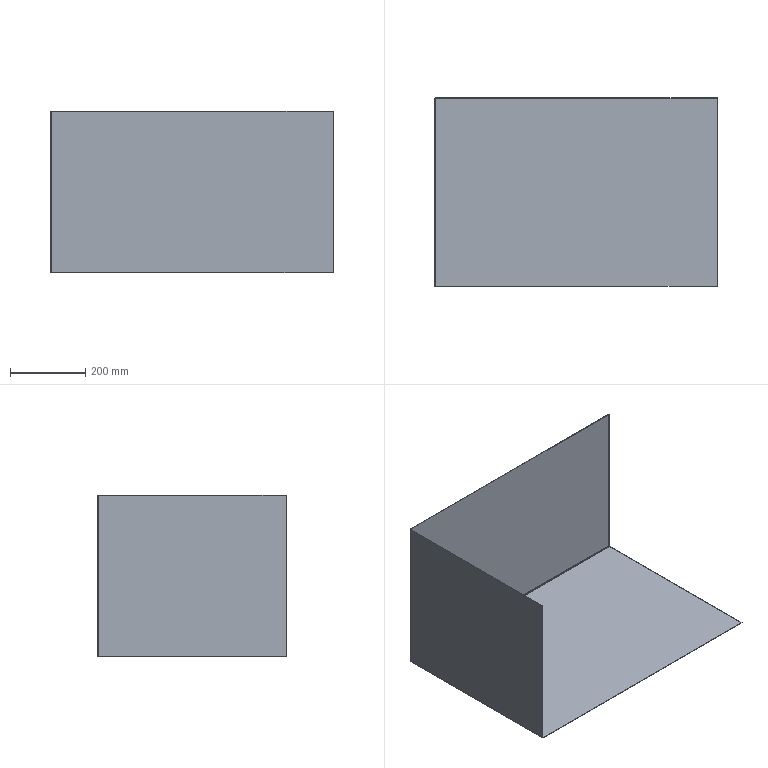Part | 1 solid | 22 faces | box 750 x 500 x 430 mm | volume 1090375 mm3 | plane 16 | cylinder 4 | spline 2 | commonest cylinder face diameters 1.473 x2 3.873 x2
STEP:
#1=CARTESIAN_POINT('',(-373.063,-250.,-1.2));
#2=VERTEX_POINT('',#1);
#3=CARTESIAN_POINT('',(-373.063,248.063,-1.2));
#4=VERTEX_POINT('',#3);
#5=CARTESIAN_POINT('',(-373.063,-250.,-1.2));
#6=DIRECTION('',(0.,1.,0.));
#7=VECTOR('',#6,1000.);
#8=LINE('',#5,#7);
#9=EDGE_CURVE('',#2,#4,#8,.T.);
#10=ORIENTED_EDGE('',*,*,#9,.T.);
#11=CARTESIAN_POINT('',(375.,248.063,-1.2));
#12=VERTEX_POINT('',#11);
#13=CARTESIAN_POINT('',(-373.093,248.063,-1.2));
#14=DIRECTION('',(1.,0.,0.));
#15=VECTOR('',#14,1000.);
#16=LINE('',#13,#15);
#17=EDGE_CURVE('',#4,#12,#16,.T.);
#18=ORIENTED_EDGE('',*,*,#17,.T.);
#19=CARTESIAN_POINT('',(375.,-250.,-1.2));
#20=VERTEX_POINT('',#19);
#21=CARTESIAN_POINT('',(375.,250.,-1.2));
#22=DIRECTION('',(0.,1.,0.));
#23=VECTOR('',#22,1000.);
#24=LINE('',#21,#23);
#25=EDGE_CURVE('',#20,#12,#24,.T.);
#26=ORIENTED_EDGE('',*,*,#25,.F.);
#27=CARTESIAN_POINT('',(-375.,-250.,-1.2));
#28=DIRECTION('',(1.,0.,0.));
#29=VECTOR('',#28,1000.);
#30=LINE('',#27,#29);
#31=EDGE_CURVE('',#2,#20,#30,.T.);
#32=ORIENTED_EDGE('',*,*,#31,.F.);
#33=EDGE_LOOP('',(#10,#18,#26,#32));
#34=FACE_OUTER_BOUND('',#33,.T.);
#35=CARTESIAN_POINT('',(0.,0.,-1.2));
#36=DIRECTION('',(0.,0.,1.));
#37=DIRECTION('',(1.,0.,0.));
#38=AXIS2_PLACEMENT_3D('',#35,#36,#37);
#39=PLANE('',#38);
#40=ADVANCED_FACE('',(#34),#39,.F.);
#41=CARTESIAN_POINT('',(-373.063,248.063,0.));
#42=VERTEX_POINT('',#41);
#43=CARTESIAN_POINT('',(375.,248.063,0.));
#44=VERTEX_POINT('',#43);
#45=CARTESIAN_POINT('',(-373.093,248.063,0.));
#46=DIRECTION('',(1.,0.,0.));
#47=VECTOR('',#46,1000.);
#48=LINE('',#45,#47);
#49=EDGE_CURVE('',#42,#44,#48,.T.);
#50=ORIENTED_EDGE('',*,*,#49,.F.);
#51=CARTESIAN_POINT('',(-373.063,-250.,0.));
#52=VERTEX_POINT('',#51);
#53=CARTESIAN_POINT('',(-373.063,-250.,0.));
#54=DIRECTION('',(0.,1.,0.));
#55=VECTOR('',#54,1000.);
#56=LINE('',#53,#55);
#57=EDGE_CURVE('',#52,#42,#56,.T.);
#58=ORIENTED_EDGE('',*,*,#57,.F.);
#59=CARTESIAN_POINT('',(375.,-250.,0.));
#60=VERTEX_POINT('',#59);
#61=CARTESIAN_POINT('',(-375.,-250.,0.));
#62=DIRECTION('',(1.,0.,0.));
#63=VECTOR('',#62,1000.);
#64=LINE('',#61,#63);
#65=EDGE_CURVE('',#52,#60,#64,.T.);
#66=ORIENTED_EDGE('',*,*,#65,.T.);
#67=CARTESIAN_POINT('',(375.,250.,0.));
#68=DIRECTION('',(0.,1.,0.));
#69=VECTOR('',#68,1000.);
#70=LINE('',#67,#69);
#71=EDGE_CURVE('',#60,#44,#70,.T.);
#72=ORIENTED_EDGE('',*,*,#71,.T.);
#73=EDGE_LOOP('',(#50,#58,#66,#72));
#74=FACE_OUTER_BOUND('',#73,.T.);
#75=CARTESIAN_POINT('',(0.,0.,0.));
#76=DIRECTION('',(0.,0.,1.));
#77=DIRECTION('',(1.,0.,0.));
#78=AXIS2_PLACEMENT_3D('',#75,#76,#77);
#79=PLANE('',#78);
#80=ADVANCED_FACE('',(#74),#79,.T.);
#81=ORIENTED_EDGE('',*,*,#65,.F.);
#82=CARTESIAN_POINT('',(-373.063,-250.,0.));
#83=DIRECTION('',(0.,0.,-1.));
#84=VECTOR('',#83,1000.);
#85=LINE('',#82,#84);
#86=EDGE_CURVE('',#52,#2,#85,.T.);
#87=ORIENTED_EDGE('',*,*,#86,.T.);
#88=ORIENTED_EDGE('',*,*,#31,.T.);
#89=CARTESIAN_POINT('',(375.,-250.,-1.2));
#90=DIRECTION('',(0.,0.,1.));
#91=VECTOR('',#90,1000.);
#92=LINE('',#89,#91);
#93=EDGE_CURVE('',#20,#60,#92,.T.);
#94=ORIENTED_EDGE('',*,*,#93,.T.);
#95=EDGE_LOOP('',(#81,#87,#88,#94));
#96=FACE_OUTER_BOUND('',#95,.T.);
#97=CARTESIAN_POINT('',(-375.,-250.,-1.2));
#98=DIRECTION('',(0.,-1.,0.));
#99=DIRECTION('',(0.,0.,-1.));
#100=AXIS2_PLACEMENT_3D('',#97,#98,#99);
#101=PLANE('',#100);
#102=ADVANCED_FACE('',(#96),#101,.T.);
#103=CARTESIAN_POINT('',(375.,248.063,0.));
#104=DIRECTION('',(0.,0.,-1.));
#105=VECTOR('',#104,1000.);
#106=LINE('',#103,#105);
#107=EDGE_CURVE('',#44,#12,#106,.T.);
#108=ORIENTED_EDGE('',*,*,#107,.F.);
#109=ORIENTED_EDGE('',*,*,#71,.F.);
#110=ORIENTED_EDGE('',*,*,#93,.F.);
#111=ORIENTED_EDGE('',*,*,#25,.T.);
#112=EDGE_LOOP('',(#108,#109,#110,#111));
#113=FACE_OUTER_BOUND('',#112,.T.);
#114=CARTESIAN_POINT('',(375.,250.,-1.2));
#115=DIRECTION('',(1.,0.,0.));
#116=DIRECTION('',(0.,1.,0.));
#117=AXIS2_PLACEMENT_3D('',#114,#115,#116);
#118=PLANE('',#117);
#119=ADVANCED_FACE('',(#113),#118,.T.);
#120=CARTESIAN_POINT('',(375.,248.8,0.7366));
#121=VERTEX_POINT('',#120);
#122=CARTESIAN_POINT('',(375.,250.,0.7366));
#123=VERTEX_POINT('',#122);
#124=CARTESIAN_POINT('',(375.,250.,0.7366));
#125=DIRECTION('',(0.,1.,0.));
#126=VECTOR('',#125,1000.);
#127=LINE('',#124,#126);
#128=EDGE_CURVE('',#121,#123,#127,.T.);
#129=ORIENTED_EDGE('',*,*,#128,.F.);
#130=CARTESIAN_POINT('',(375.,248.063,0.7366));
#131=DIRECTION('',(1.,0.,0.));
#132=DIRECTION('',(0.,0.,1.));
#133=AXIS2_PLACEMENT_3D('',#130,#131,#132);
#134=CIRCLE('',#133,0.7366);
#135=EDGE_CURVE('',#44,#121,#134,.T.);
#136=ORIENTED_EDGE('',*,*,#135,.F.);
#137=ORIENTED_EDGE('',*,*,#107,.T.);
#138=CARTESIAN_POINT('',(375.,248.063,0.7366));
#139=DIRECTION('',(1.,0.,0.));
#140=DIRECTION('',(0.,0.,1.));
#141=AXIS2_PLACEMENT_3D('',#138,#139,#140);
#142=CIRCLE('',#141,1.937);
#143=EDGE_CURVE('',#12,#123,#142,.T.);
#144=ORIENTED_EDGE('',*,*,#143,.T.);
#145=EDGE_LOOP('',(#129,#136,#137,#144));
#146=FACE_OUTER_BOUND('',#145,.T.);
#147=CARTESIAN_POINT('',(375.,248.063,0.7366));
#148=DIRECTION('',(1.,0.,0.));
#149=DIRECTION('',(0.,0.,-1.));
#150=AXIS2_PLACEMENT_3D('',#147,#148,#149);
#151=PLANE('',#150);
#152=ADVANCED_FACE('',(#146),#151,.T.);
#153=CARTESIAN_POINT('',(-373.093,248.8,0.7366));
#154=VERTEX_POINT('',#153);
#155=CARTESIAN_POINT('',(-373.093,248.8,0.7366));
#156=CARTESIAN_POINT('',(-373.088,248.8,0.5438));
#157=CARTESIAN_POINT('',(-373.083,248.721,0.3521));
#158=CARTESIAN_POINT('',(-373.073,248.448,0.07939));
#159=CARTESIAN_POINT('',(-373.068,248.256,0.));
#160=CARTESIAN_POINT('',(-373.063,248.063,0.));
#161=B_SPLINE_CURVE_WITH_KNOTS('',3,(#155,#156,#157,#158,#159,#160),.UNSPECIFIED.,.F.,.F.,(4,2,4),(0.,0.5,1.),.UNSPECIFIED.);
#162=EDGE_CURVE('',#154,#42,#161,.T.);
#163=ORIENTED_EDGE('',*,*,#162,.F.);
#164=CARTESIAN_POINT('',(-373.093,250.,0.7366));
#165=VERTEX_POINT('',#164);
#166=CARTESIAN_POINT('',(-373.093,248.8,0.7366));
#167=DIRECTION('',(0.,-1.,0.));
#168=VECTOR('',#167,1000.);
#169=LINE('',#166,#168);
#170=EDGE_CURVE('',#165,#154,#169,.T.);
#171=ORIENTED_EDGE('',*,*,#170,.F.);
#172=CARTESIAN_POINT('',(-373.093,250.,0.7366));
#173=CARTESIAN_POINT('',(-373.09,250.,0.4831));
#174=CARTESIAN_POINT('',(-373.088,249.95,0.2297));
#175=CARTESIAN_POINT('',(-373.083,249.756,-0.2387));
#176=CARTESIAN_POINT('',(-373.081,249.612,-0.4535));
#177=CARTESIAN_POINT('',(-373.076,249.254,-0.812));
#178=CARTESIAN_POINT('',(-373.073,249.039,-0.9556));
#179=CARTESIAN_POINT('',(-373.068,248.57,-1.15));
#180=CARTESIAN_POINT('',(-373.066,248.317,-1.2));
#181=CARTESIAN_POINT('',(-373.063,248.063,-1.2));
#182=B_SPLINE_CURVE_WITH_KNOTS('',3,(#172,#173,#174,#175,#176,#177,#178,#179,#180,#181),.UNSPECIFIED.,.F.,.F.,(4,2,2,2,4),(0.,0.25,0.5,0.75,1.),.UNSPECIFIED.);
#183=EDGE_CURVE('',#165,#4,#182,.T.);
#184=ORIENTED_EDGE('',*,*,#183,.T.);
#185=CARTESIAN_POINT('',(-373.063,248.063,0.));
#186=DIRECTION('',(0.,0.,-1.));
#187=VECTOR('',#186,1000.);
#188=LINE('',#185,#187);
#189=EDGE_CURVE('',#42,#4,#188,.T.);
#190=ORIENTED_EDGE('',*,*,#189,.F.);
#191=EDGE_LOOP('',(#163,#171,#184,#190));
#192=FACE_OUTER_BOUND('',#191,.T.);
#193=CARTESIAN_POINT('',(-373.093,250.012,0.7366));
#194=CARTESIAN_POINT('',(-373.09,250.012,0.4815));
#195=CARTESIAN_POINT('',(-373.088,249.961,0.2266));
#196=CARTESIAN_POINT('',(-373.083,249.766,-0.2448));
#197=CARTESIAN_POINT('',(-373.081,249.622,-0.4609));
#198=CARTESIAN_POINT('',(-373.076,249.261,-0.8216));
#199=CARTESIAN_POINT('',(-373.073,249.045,-0.9661));
#200=CARTESIAN_POINT('',(-373.068,248.573,-1.161));
#201=CARTESIAN_POINT('',(-373.066,248.319,-1.212));
#202=CARTESIAN_POINT('',(-373.063,248.063,-1.212));
#203=CARTESIAN_POINT('',(-373.093,250.,0.7366));
#204=CARTESIAN_POINT('',(-373.09,250.,0.4831));
#205=CARTESIAN_POINT('',(-373.088,249.95,0.2297));
#206=CARTESIAN_POINT('',(-373.083,249.756,-0.2387));
#207=CARTESIAN_POINT('',(-373.081,249.612,-0.4535));
#208=CARTESIAN_POINT('',(-373.076,249.254,-0.812));
#209=CARTESIAN_POINT('',(-373.073,249.039,-0.9556));
#210=CARTESIAN_POINT('',(-373.068,248.57,-1.15));
#211=CARTESIAN_POINT('',(-373.066,248.317,-1.2));
#212=CARTESIAN_POINT('',(-373.063,248.063,-1.2));
#213=CARTESIAN_POINT('',(-373.093,248.8,0.7366));
#214=CARTESIAN_POINT('',(-373.09,248.8,0.6402));
#215=CARTESIAN_POINT('',(-373.088,248.781,0.5438));
#216=CARTESIAN_POINT('',(-373.083,248.707,0.3656));
#217=CARTESIAN_POINT('',(-373.081,248.652,0.2839));
#218=CARTESIAN_POINT('',(-373.076,248.516,0.1476));
#219=CARTESIAN_POINT('',(-373.073,248.434,0.09297));
#220=CARTESIAN_POINT('',(-373.068,248.256,0.01917));
#221=CARTESIAN_POINT('',(-373.066,248.16,0.));
#222=CARTESIAN_POINT('',(-373.063,248.063,0.));
#223=CARTESIAN_POINT('',(-373.093,248.788,0.7366));
#224=CARTESIAN_POINT('',(-373.09,248.788,0.6417));
#225=CARTESIAN_POINT('',(-373.088,248.769,0.547));
#226=CARTESIAN_POINT('',(-373.083,248.696,0.3717));
#227=CARTESIAN_POINT('',(-373.081,248.643,0.2914));
#228=CARTESIAN_POINT('',(-373.076,248.509,0.1573));
#229=CARTESIAN_POINT('',(-373.073,248.428,0.1036));
#230=CARTESIAN_POINT('',(-373.068,248.253,0.03098));
#231=CARTESIAN_POINT('',(-373.066,248.158,0.01212));
#232=CARTESIAN_POINT('',(-373.063,248.063,0.01212));
#233=B_SPLINE_SURFACE_WITH_KNOTS('',1,3,((#193,#194,#195,#196,#197,#198,#199,#200,#201,#202),(#203,#204,#205,#206,#207,#208,#209,#210,#211,#212),(#213,#214,#215,#216,#217,#218,#219,#220,#221,#222),(#223,#224,#225,#226,#227,#228,#229,#230,#231,#232)),.UNSPECIFIED.,.F.,.F.,.F.,(2,1,1,2),(4,2,2,2,4),(-0.01,0.,1.,1.01),(0.,0.25,0.5,0.75,1.),.UNSPECIFIED.);
#234=ADVANCED_FACE('',(#192),#233,.F.);
#235=ORIENTED_EDGE('',*,*,#17,.F.);
#236=ORIENTED_EDGE('',*,*,#183,.F.);
#237=CARTESIAN_POINT('',(0.,250.,0.7366));
#238=DIRECTION('',(-1.,0.,0.));
#239=VECTOR('',#238,1000.);
#240=LINE('',#237,#239);
#241=EDGE_CURVE('',#123,#165,#240,.T.);
#242=ORIENTED_EDGE('',*,*,#241,.F.);
#243=ORIENTED_EDGE('',*,*,#143,.F.);
#244=EDGE_LOOP('',(#235,#236,#242,#243));
#245=FACE_OUTER_BOUND('',#244,.T.);
#246=CARTESIAN_POINT('',(-373.093,248.063,0.7366));
#247=DIRECTION('',(-1.,0.,0.));
#248=DIRECTION('',(0.,1.,0.));
#249=AXIS2_PLACEMENT_3D('',#246,#247,#248);
#250=CYLINDRICAL_SURFACE('',#249,1.937);
#251=ADVANCED_FACE('',(#245),#250,.T.);
#252=ORIENTED_EDGE('',*,*,#49,.T.);
#253=ORIENTED_EDGE('',*,*,#135,.T.);
#254=CARTESIAN_POINT('',(375.,248.8,0.7366));
#255=DIRECTION('',(-1.,0.,0.));
#256=VECTOR('',#255,1000.);
#257=LINE('',#254,#256);
#258=EDGE_CURVE('',#121,#154,#257,.T.);
#259=ORIENTED_EDGE('',*,*,#258,.T.);
#260=ORIENTED_EDGE('',*,*,#162,.T.);
#261=EDGE_LOOP('',(#252,#253,#259,#260));
#262=FACE_OUTER_BOUND('',#261,.T.);
#263=CARTESIAN_POINT('',(-373.093,248.063,0.7366));
#264=DIRECTION('',(-1.,0.,0.));
#265=DIRECTION('',(0.,1.,0.));
#266=AXIS2_PLACEMENT_3D('',#263,#264,#265);
#267=CYLINDRICAL_SURFACE('',#266,0.7366);
#268=ADVANCED_FACE('',(#262),#267,.F.);
#269=CARTESIAN_POINT('',(375.,248.8,428.8));
#270=VERTEX_POINT('',#269);
#271=CARTESIAN_POINT('',(375.,248.8,0.));
#272=DIRECTION('',(0.,0.,1.));
#273=VECTOR('',#272,1000.);
#274=LINE('',#271,#273);
#275=EDGE_CURVE('',#121,#270,#274,.T.);
#276=ORIENTED_EDGE('',*,*,#275,.F.);
#277=ORIENTED_EDGE('',*,*,#128,.T.);
#278=CARTESIAN_POINT('',(375.,250.,428.8));
#279=VERTEX_POINT('',#278);
#280=CARTESIAN_POINT('',(375.,250.,428.8));
#281=DIRECTION('',(0.,0.,1.));
#282=VECTOR('',#281,1000.);
#283=LINE('',#280,#282);
#284=EDGE_CURVE('',#123,#279,#283,.T.);
#285=ORIENTED_EDGE('',*,*,#284,.T.);
#286=CARTESIAN_POINT('',(375.,250.,428.8));
#287=DIRECTION('',(0.,-1.,0.));
#288=VECTOR('',#287,1000.);
#289=LINE('',#286,#288);
#290=EDGE_CURVE('',#279,#270,#289,.T.);
#291=ORIENTED_EDGE('',*,*,#290,.T.);
#292=EDGE_LOOP('',(#276,#277,#285,#291));
#293=FACE_OUTER_BOUND('',#292,.T.);
#294=CARTESIAN_POINT('',(375.,250.,428.8));
#295=DIRECTION('',(1.,0.,0.));
#296=DIRECTION('',(0.,0.,-1.));
#297=AXIS2_PLACEMENT_3D('',#294,#295,#296);
#298=PLANE('',#297);
#299=ADVANCED_FACE('',(#293),#298,.T.);
#300=CARTESIAN_POINT('',(-373.093,250.,428.8));
#301=VERTEX_POINT('',#300);
#302=CARTESIAN_POINT('',(-373.093,250.,0.));
#303=DIRECTION('',(0.,0.,-1.));
#304=VECTOR('',#303,1000.);
#305=LINE('',#302,#304);
#306=EDGE_CURVE('',#301,#165,#305,.T.);
#307=ORIENTED_EDGE('',*,*,#306,.F.);
#308=CARTESIAN_POINT('',(-375.,250.,428.8));
#309=DIRECTION('',(-1.,0.,0.));
#310=VECTOR('',#309,1000.);
#311=LINE('',#308,#310);
#312=EDGE_CURVE('',#279,#301,#311,.T.);
#313=ORIENTED_EDGE('',*,*,#312,.F.);
#314=ORIENTED_EDGE('',*,*,#284,.F.);
#315=ORIENTED_EDGE('',*,*,#241,.T.);
#316=EDGE_LOOP('',(#307,#313,#314,#315));
#317=FACE_OUTER_BOUND('',#316,.T.);
#318=CARTESIAN_POINT('',(0.,250.,0.));
#319=DIRECTION('',(0.,1.,0.));
#320=DIRECTION('',(0.,0.,1.));
#321=AXIS2_PLACEMENT_3D('',#318,#319,#320);
#322=PLANE('',#321);
#323=ADVANCED_FACE('',(#317),#322,.T.);
#324=CARTESIAN_POINT('',(-373.093,248.8,428.8));
#325=VERTEX_POINT('',#324);
#326=CARTESIAN_POINT('',(0.,248.8,428.8));
#327=DIRECTION('',(-1.,0.,0.));
#328=VECTOR('',#327,1000.);
#329=LINE('',#326,#328);
#330=EDGE_CURVE('',#270,#325,#329,.T.);
#331=ORIENTED_EDGE('',*,*,#330,.T.);
#332=CARTESIAN_POINT('',(-373.093,248.8,0.));
#333=DIRECTION('',(0.,0.,1.));
#334=VECTOR('',#333,1000.);
#335=LINE('',#332,#334);
#336=EDGE_CURVE('',#154,#325,#335,.T.);
#337=ORIENTED_EDGE('',*,*,#336,.F.);
#338=ORIENTED_EDGE('',*,*,#258,.F.);
#339=ORIENTED_EDGE('',*,*,#275,.T.);
#340=EDGE_LOOP('',(#331,#337,#338,#339));
#341=FACE_OUTER_BOUND('',#340,.T.);
#342=CARTESIAN_POINT('',(0.,248.8,0.));
#343=DIRECTION('',(0.,1.,0.));
#344=DIRECTION('',(0.,0.,1.));
#345=AXIS2_PLACEMENT_3D('',#342,#343,#344);
#346=PLANE('',#345);
#347=ADVANCED_FACE('',(#341),#346,.F.);
#348=CARTESIAN_POINT('',(-373.093,248.8,428.8));
#349=DIRECTION('',(0.,1.,0.));
#350=VECTOR('',#349,1000.);
#351=LINE('',#348,#350);
#352=EDGE_CURVE('',#325,#301,#351,.T.);
#353=ORIENTED_EDGE('',*,*,#352,.F.);
#354=ORIENTED_EDGE('',*,*,#330,.F.);
#355=ORIENTED_EDGE('',*,*,#290,.F.);
#356=ORIENTED_EDGE('',*,*,#312,.T.);
#357=EDGE_LOOP('',(#353,#354,#355,#356));
#358=FACE_OUTER_BOUND('',#357,.T.);
#359=CARTESIAN_POINT('',(-375.,250.,428.8));
#360=DIRECTION('',(0.,0.,1.));
#361=DIRECTION('',(0.,-1.,0.));
#362=AXIS2_PLACEMENT_3D('',#359,#360,#361);
#363=PLANE('',#362);
#364=ADVANCED_FACE('',(#358),#363,.T.);
#365=ORIENTED_EDGE('',*,*,#336,.T.);
#366=ORIENTED_EDGE('',*,*,#352,.T.);
#367=ORIENTED_EDGE('',*,*,#306,.T.);
#368=ORIENTED_EDGE('',*,*,#170,.T.);
#369=EDGE_LOOP('',(#365,#366,#367,#368));
#370=FACE_OUTER_BOUND('',#369,.T.);
#371=CARTESIAN_POINT('',(-373.093,248.8,0.));
#372=DIRECTION('',(1.,0.,0.));
#373=DIRECTION('',(0.,0.,-1.));
#374=AXIS2_PLACEMENT_3D('',#371,#372,#373);
#375=PLANE('',#374);
#376=ADVANCED_FACE('',(#370),#375,.F.);
#377=CARTESIAN_POINT('',(-375.,248.093,0.7366));
#378=VERTEX_POINT('',#377);
#379=CARTESIAN_POINT('',(-373.8,248.093,0.7366));
#380=VERTEX_POINT('',#379);
#381=CARTESIAN_POINT('',(-373.8,248.093,0.7366));
#382=DIRECTION('',(1.,0.,0.));
#383=VECTOR('',#382,1000.);
#384=LINE('',#381,#383);
#385=EDGE_CURVE('',#378,#380,#384,.T.);
#386=ORIENTED_EDGE('',*,*,#385,.T.);
#387=CARTESIAN_POINT('',(-373.063,248.063,0.));
#388=CARTESIAN_POINT('',(-373.256,248.068,0.));
#389=CARTESIAN_POINT('',(-373.448,248.073,0.07939));
#390=CARTESIAN_POINT('',(-373.721,248.083,0.3521));
#391=CARTESIAN_POINT('',(-373.8,248.088,0.5438));
#392=CARTESIAN_POINT('',(-373.8,248.093,0.7366));
#393=B_SPLINE_CURVE_WITH_KNOTS('',3,(#387,#388,#389,#390,#391,#392),.UNSPECIFIED.,.F.,.F.,(4,2,4),(0.,0.5,1.),.UNSPECIFIED.);
#394=EDGE_CURVE('',#42,#380,#393,.T.);
#395=ORIENTED_EDGE('',*,*,#394,.F.);
#396=ORIENTED_EDGE('',*,*,#189,.T.);
#397=CARTESIAN_POINT('',(-373.063,248.063,-1.2));
#398=CARTESIAN_POINT('',(-373.317,248.066,-1.2));
#399=CARTESIAN_POINT('',(-373.57,248.068,-1.15));
#400=CARTESIAN_POINT('',(-374.039,248.073,-0.9556));
#401=CARTESIAN_POINT('',(-374.254,248.076,-0.812));
#402=CARTESIAN_POINT('',(-374.612,248.081,-0.4535));
#403=CARTESIAN_POINT('',(-374.756,248.083,-0.2387));
#404=CARTESIAN_POINT('',(-374.95,248.088,0.2297));
#405=CARTESIAN_POINT('',(-375.,248.09,0.4831));
#406=CARTESIAN_POINT('',(-375.,248.093,0.7366));
#407=B_SPLINE_CURVE_WITH_KNOTS('',3,(#397,#398,#399,#400,#401,#402,#403,#404,#405,#406),.UNSPECIFIED.,.F.,.F.,(4,2,2,2,4),(0.,0.25,0.5,0.75,1.),.UNSPECIFIED.);
#408=EDGE_CURVE('',#4,#378,#407,.T.);
#409=ORIENTED_EDGE('',*,*,#408,.T.);
#410=EDGE_LOOP('',(#386,#395,#396,#409));
#411=FACE_OUTER_BOUND('',#410,.T.);
#412=CARTESIAN_POINT('',(-373.063,248.063,-1.212));
#413=CARTESIAN_POINT('',(-373.319,248.066,-1.212));
#414=CARTESIAN_POINT('',(-373.573,248.068,-1.161));
#415=CARTESIAN_POINT('',(-374.045,248.073,-0.9661));
#416=CARTESIAN_POINT('',(-374.261,248.076,-0.8216));
#417=CARTESIAN_POINT('',(-374.622,248.081,-0.4609));
#418=CARTESIAN_POINT('',(-374.766,248.083,-0.2448));
#419=CARTESIAN_POINT('',(-374.961,248.088,0.2266));
#420=CARTESIAN_POINT('',(-375.012,248.09,0.4815));
#421=CARTESIAN_POINT('',(-375.012,248.093,0.7366));
#422=CARTESIAN_POINT('',(-373.063,248.063,-1.2));
#423=CARTESIAN_POINT('',(-373.317,248.066,-1.2));
#424=CARTESIAN_POINT('',(-373.57,248.068,-1.15));
#425=CARTESIAN_POINT('',(-374.039,248.073,-0.9556));
#426=CARTESIAN_POINT('',(-374.254,248.076,-0.812));
#427=CARTESIAN_POINT('',(-374.612,248.081,-0.4535));
#428=CARTESIAN_POINT('',(-374.756,248.083,-0.2387));
#429=CARTESIAN_POINT('',(-374.95,248.088,0.2297));
#430=CARTESIAN_POINT('',(-375.,248.09,0.4831));
#431=CARTESIAN_POINT('',(-375.,248.093,0.7366));
#432=CARTESIAN_POINT('',(-373.063,248.063,0.));
#433=CARTESIAN_POINT('',(-373.16,248.066,0.));
#434=CARTESIAN_POINT('',(-373.256,248.068,0.01917));
#435=CARTESIAN_POINT('',(-373.434,248.073,0.09297));
#436=CARTESIAN_POINT('',(-373.516,248.076,0.1476));
#437=CARTESIAN_POINT('',(-373.652,248.081,0.2839));
#438=CARTESIAN_POINT('',(-373.707,248.083,0.3656));
#439=CARTESIAN_POINT('',(-373.781,248.088,0.5438));
#440=CARTESIAN_POINT('',(-373.8,248.09,0.6402));
#441=CARTESIAN_POINT('',(-373.8,248.093,0.7366));
#442=CARTESIAN_POINT('',(-373.063,248.063,0.01212));
#443=CARTESIAN_POINT('',(-373.158,248.066,0.01212));
#444=CARTESIAN_POINT('',(-373.253,248.068,0.03098));
#445=CARTESIAN_POINT('',(-373.428,248.073,0.1036));
#446=CARTESIAN_POINT('',(-373.509,248.076,0.1573));
#447=CARTESIAN_POINT('',(-373.643,248.081,0.2914));
#448=CARTESIAN_POINT('',(-373.696,248.083,0.3717));
#449=CARTESIAN_POINT('',(-373.769,248.088,0.547));
#450=CARTESIAN_POINT('',(-373.788,248.09,0.6417));
#451=CARTESIAN_POINT('',(-373.788,248.093,0.7366));
#452=B_SPLINE_SURFACE_WITH_KNOTS('',1,3,((#412,#413,#414,#415,#416,#417,#418,#419,#420,#421),(#422,#423,#424,#425,#426,#427,#428,#429,#430,#431),(#432,#433,#434,#435,#436,#437,#438,#439,#440,#441),(#442,#443,#444,#445,#446,#447,#448,#449,#450,#451)),.UNSPECIFIED.,.F.,.F.,.F.,(2,1,1,2),(4,2,2,2,4),(-0.01,0.,1.,1.01),(0.,0.25,0.5,0.75,1.),.UNSPECIFIED.);
#453=ADVANCED_FACE('',(#411),#452,.F.);
#454=CARTESIAN_POINT('',(-373.8,-250.,0.7366));
#455=VERTEX_POINT('',#454);
#456=CARTESIAN_POINT('',(-373.063,-250.,0.7366));
#457=DIRECTION('',(0.,-1.,0.));
#458=DIRECTION('',(0.,0.,-1.));
#459=AXIS2_PLACEMENT_3D('',#456,#457,#458);
#460=CIRCLE('',#459,0.7366);
#461=EDGE_CURVE('',#455,#52,#460,.T.);
#462=ORIENTED_EDGE('',*,*,#461,.F.);
#463=CARTESIAN_POINT('',(-375.,-250.,0.7366));
#464=VERTEX_POINT('',#463);
#465=CARTESIAN_POINT('',(-373.8,-250.,0.7366));
#466=DIRECTION('',(-1.,0.,0.));
#467=VECTOR('',#466,1000.);
#468=LINE('',#465,#467);
#469=EDGE_CURVE('',#455,#464,#468,.T.);
#470=ORIENTED_EDGE('',*,*,#469,.T.);
#471=CARTESIAN_POINT('',(-373.063,-250.,0.7366));
#472=DIRECTION('',(0.,-1.,0.));
#473=DIRECTION('',(0.,0.,-1.));
#474=AXIS2_PLACEMENT_3D('',#471,#472,#473);
#475=CIRCLE('',#474,1.937);
#476=EDGE_CURVE('',#464,#2,#475,.T.);
#477=ORIENTED_EDGE('',*,*,#476,.T.);
#478=ORIENTED_EDGE('',*,*,#86,.F.);
#479=EDGE_LOOP('',(#462,#470,#477,#478));
#480=FACE_OUTER_BOUND('',#479,.T.);
#481=CARTESIAN_POINT('',(-373.063,-250.,0.7366));
#482=DIRECTION('',(0.,1.,0.));
#483=DIRECTION('',(0.,0.,1.));
#484=AXIS2_PLACEMENT_3D('',#481,#482,#483);
#485=PLANE('',#484);
#486=ADVANCED_FACE('',(#480),#485,.F.);
#487=ORIENTED_EDGE('',*,*,#9,.F.);
#488=ORIENTED_EDGE('',*,*,#476,.F.);
#489=CARTESIAN_POINT('',(-375.,250.,0.7366));
#490=DIRECTION('',(0.,1.,0.));
#491=VECTOR('',#490,1000.);
#492=LINE('',#489,#491);
#493=EDGE_CURVE('',#464,#378,#492,.T.);
#494=ORIENTED_EDGE('',*,*,#493,.T.);
#495=ORIENTED_EDGE('',*,*,#408,.F.);
#496=EDGE_LOOP('',(#487,#488,#494,#495));
#497=FACE_OUTER_BOUND('',#496,.T.);
#498=CARTESIAN_POINT('',(-373.063,-250.,0.7366));
#499=DIRECTION('',(0.,-1.,0.));
#500=DIRECTION('',(-1.,0.,0.));
#501=AXIS2_PLACEMENT_3D('',#498,#499,#500);
#502=CYLINDRICAL_SURFACE('',#501,1.937);
#503=ADVANCED_FACE('',(#497),#502,.T.);
#504=ORIENTED_EDGE('',*,*,#57,.T.);
#505=ORIENTED_EDGE('',*,*,#394,.T.);
#506=CARTESIAN_POINT('',(-373.8,250.,0.7366));
#507=DIRECTION('',(0.,-1.,0.));
#508=VECTOR('',#507,1000.);
#509=LINE('',#506,#508);
#510=EDGE_CURVE('',#380,#455,#509,.T.);
#511=ORIENTED_EDGE('',*,*,#510,.T.);
#512=ORIENTED_EDGE('',*,*,#461,.T.);
#513=EDGE_LOOP('',(#504,#505,#511,#512));
#514=FACE_OUTER_BOUND('',#513,.T.);
#515=CARTESIAN_POINT('',(-373.063,-250.,0.7366));
#516=DIRECTION('',(0.,-1.,0.));
#517=DIRECTION('',(-1.,0.,0.));
#518=AXIS2_PLACEMENT_3D('',#515,#516,#517);
#519=CYLINDRICAL_SURFACE('',#518,0.7366);
#520=ADVANCED_FACE('',(#514),#519,.F.);
#521=CARTESIAN_POINT('',(-373.8,248.093,428.8));
#522=VERTEX_POINT('',#521);
#523=CARTESIAN_POINT('',(-375.,248.093,428.8));
#524=VERTEX_POINT('',#523);
#525=CARTESIAN_POINT('',(-375.,248.093,428.8));
#526=DIRECTION('',(-1.,0.,0.));
#527=VECTOR('',#526,1000.);
#528=LINE('',#525,#527);
#529=EDGE_CURVE('',#522,#524,#528,.T.);
#530=ORIENTED_EDGE('',*,*,#529,.F.);
#531=CARTESIAN_POINT('',(-373.8,248.093,0.));
#532=DIRECTION('',(0.,0.,1.));
#533=VECTOR('',#532,1000.);
#534=LINE('',#531,#533);
#535=EDGE_CURVE('',#380,#522,#534,.T.);
#536=ORIENTED_EDGE('',*,*,#535,.F.);
#537=ORIENTED_EDGE('',*,*,#385,.F.);
#538=CARTESIAN_POINT('',(-375.,248.093,0.));
#539=DIRECTION('',(0.,0.,1.));
#540=VECTOR('',#539,1000.);
#541=LINE('',#538,#540);
#542=EDGE_CURVE('',#378,#524,#541,.T.);
#543=ORIENTED_EDGE('',*,*,#542,.T.);
#544=EDGE_LOOP('',(#530,#536,#537,#543));
#545=FACE_OUTER_BOUND('',#544,.T.);
#546=CARTESIAN_POINT('',(-373.8,248.093,0.));
#547=DIRECTION('',(0.,1.,0.));
#548=DIRECTION('',(0.,0.,1.));
#549=AXIS2_PLACEMENT_3D('',#546,#547,#548);
#550=PLANE('',#549);
#551=ADVANCED_FACE('',(#545),#550,.T.);
#552=ORIENTED_EDGE('',*,*,#542,.F.);
#553=ORIENTED_EDGE('',*,*,#493,.F.);
#554=CARTESIAN_POINT('',(-375.,-250.,428.8));
#555=VERTEX_POINT('',#554);
#556=CARTESIAN_POINT('',(-375.,-250.,428.8));
#557=DIRECTION('',(0.,0.,-1.));
#558=VECTOR('',#557,1000.);
#559=LINE('',#556,#558);
#560=EDGE_CURVE('',#555,#464,#559,.T.);
#561=ORIENTED_EDGE('',*,*,#560,.F.);
#562=CARTESIAN_POINT('',(-375.,250.,428.8));
#563=DIRECTION('',(0.,-1.,0.));
#564=VECTOR('',#563,1000.);
#565=LINE('',#562,#564);
#566=EDGE_CURVE('',#524,#555,#565,.T.);
#567=ORIENTED_EDGE('',*,*,#566,.F.);
#568=EDGE_LOOP('',(#552,#553,#561,#567));
#569=FACE_OUTER_BOUND('',#568,.T.);
#570=CARTESIAN_POINT('',(-375.,0.,0.));
#571=DIRECTION('',(1.,0.,0.));
#572=DIRECTION('',(0.,0.,-1.));
#573=AXIS2_PLACEMENT_3D('',#570,#571,#572);
#574=PLANE('',#573);
#575=ADVANCED_FACE('',(#569),#574,.F.);
#576=ORIENTED_EDGE('',*,*,#510,.F.);
#577=ORIENTED_EDGE('',*,*,#535,.T.);
#578=CARTESIAN_POINT('',(-373.8,-250.,428.8));
#579=VERTEX_POINT('',#578);
#580=CARTESIAN_POINT('',(-373.8,0.,428.8));
#581=DIRECTION('',(0.,-1.,0.));
#582=VECTOR('',#581,1000.);
#583=LINE('',#580,#582);
#584=EDGE_CURVE('',#522,#579,#583,.T.);
#585=ORIENTED_EDGE('',*,*,#584,.T.);
#586=CARTESIAN_POINT('',(-373.8,-250.,0.));
#587=DIRECTION('',(0.,0.,-1.));
#588=VECTOR('',#587,1000.);
#589=LINE('',#586,#588);
#590=EDGE_CURVE('',#579,#455,#589,.T.);
#591=ORIENTED_EDGE('',*,*,#590,.T.);
#592=EDGE_LOOP('',(#576,#577,#585,#591));
#593=FACE_OUTER_BOUND('',#592,.T.);
#594=CARTESIAN_POINT('',(-373.8,0.,0.));
#595=DIRECTION('',(1.,0.,0.));
#596=DIRECTION('',(0.,0.,-1.));
#597=AXIS2_PLACEMENT_3D('',#594,#595,#596);
#598=PLANE('',#597);
#599=ADVANCED_FACE('',(#593),#598,.T.);
#600=ORIENTED_EDGE('',*,*,#584,.F.);
#601=ORIENTED_EDGE('',*,*,#529,.T.);
#602=ORIENTED_EDGE('',*,*,#566,.T.);
#603=CARTESIAN_POINT('',(-375.,-250.,428.8));
#604=DIRECTION('',(1.,0.,0.));
#605=VECTOR('',#604,1000.);
#606=LINE('',#603,#605);
#607=EDGE_CURVE('',#555,#579,#606,.T.);
#608=ORIENTED_EDGE('',*,*,#607,.T.);
#609=EDGE_LOOP('',(#600,#601,#602,#608));
#610=FACE_OUTER_BOUND('',#609,.T.);
#611=CARTESIAN_POINT('',(-375.,250.,428.8));
#612=DIRECTION('',(0.,0.,1.));
#613=DIRECTION('',(1.,0.,0.));
#614=AXIS2_PLACEMENT_3D('',#611,#612,#613);
#615=PLANE('',#614);
#616=ADVANCED_FACE('',(#610),#615,.T.);
#617=ORIENTED_EDGE('',*,*,#560,.T.);
#618=ORIENTED_EDGE('',*,*,#469,.F.);
#619=ORIENTED_EDGE('',*,*,#590,.F.);
#620=ORIENTED_EDGE('',*,*,#607,.F.);
#621=EDGE_LOOP('',(#617,#618,#619,#620));
#622=FACE_OUTER_BOUND('',#621,.T.);
#623=CARTESIAN_POINT('',(-375.,-250.,428.8));
#624=DIRECTION('',(0.,-1.,0.));
#625=DIRECTION('',(1.,0.,0.));
#626=AXIS2_PLACEMENT_3D('',#623,#624,#625);
#627=PLANE('',#626);
#628=ADVANCED_FACE('',(#622),#627,.T.);
#629=CLOSED_SHELL('',(#40,#80,#102,#119,#152,#234,#251,#268,#299,#323,#347,#364,#376,#453,#486,#503,#520,#551,#575,#599,#616,#628));
#630=MANIFOLD_SOLID_BREP('',#629);
#631=CARTESIAN_POINT('',(0.,0.,0.));
#632=DIRECTION('',(0.,0.,1.));
#633=DIRECTION('',(1.,0.,0.));
#634=AXIS2_PLACEMENT_3D('',#631,#632,#633);
#635=(LENGTH_UNIT()NAMED_UNIT(*)SI_UNIT(.MILLI.,.METRE.));
#636=UNCERTAINTY_MEASURE_WITH_UNIT(LENGTH_MEASURE(0.00001),#635,'','');
#637=(NAMED_UNIT(*)PLANE_ANGLE_UNIT()SI_UNIT($,.RADIAN.));
#638=(NAMED_UNIT(*)SI_UNIT($,.STERADIAN.)SOLID_ANGLE_UNIT());
#639=(GEOMETRIC_REPRESENTATION_CONTEXT(3)GLOBAL_UNCERTAINTY_ASSIGNED_CONTEXT((#636))GLOBAL_UNIT_ASSIGNED_CONTEXT((#635,#637,#638))REPRESENTATION_CONTEXT('',''));
#640=ADVANCED_BREP_SHAPE_REPRESENTATION('',(#630,#634),#639);